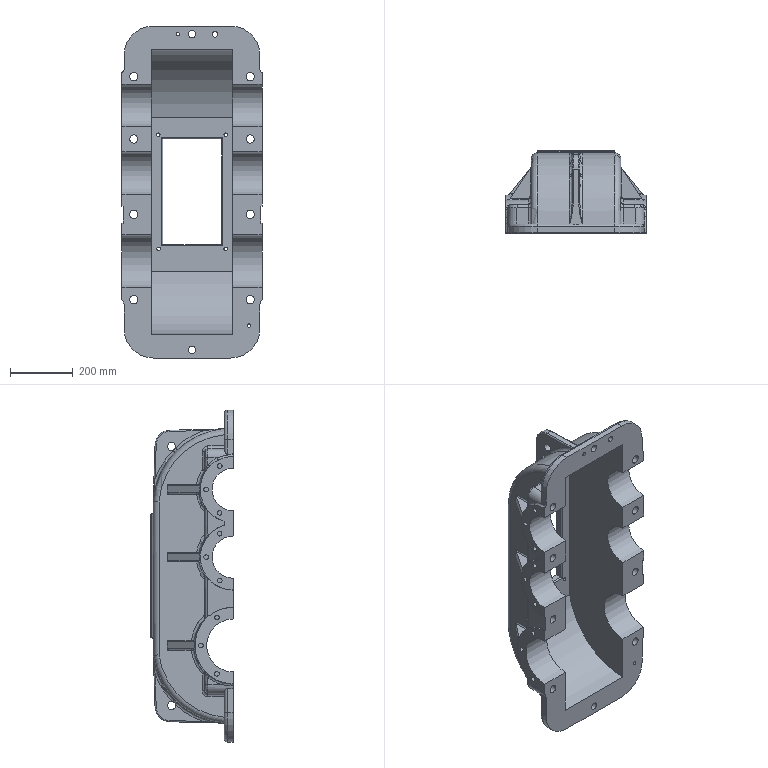Part | SolidWorks | features Fillet 30, ICE 30, MirrorPattern 4, RevCut 3, Revolution 3, Sculpt 2, Extrusion 1, Scale 1 | 1 solid | 388 faces | box 446.25 x 262.5 x 1058 mm | volume 19685797 mm3 | cylinder 156 | plane 100 | spline 77 | torus 40 | cone 11 | sphere 4 | commonest cylinder face diameters 15 x36 18.75 x28 7.5 x26 26.25 x20 11.25 x12 22.5 x4